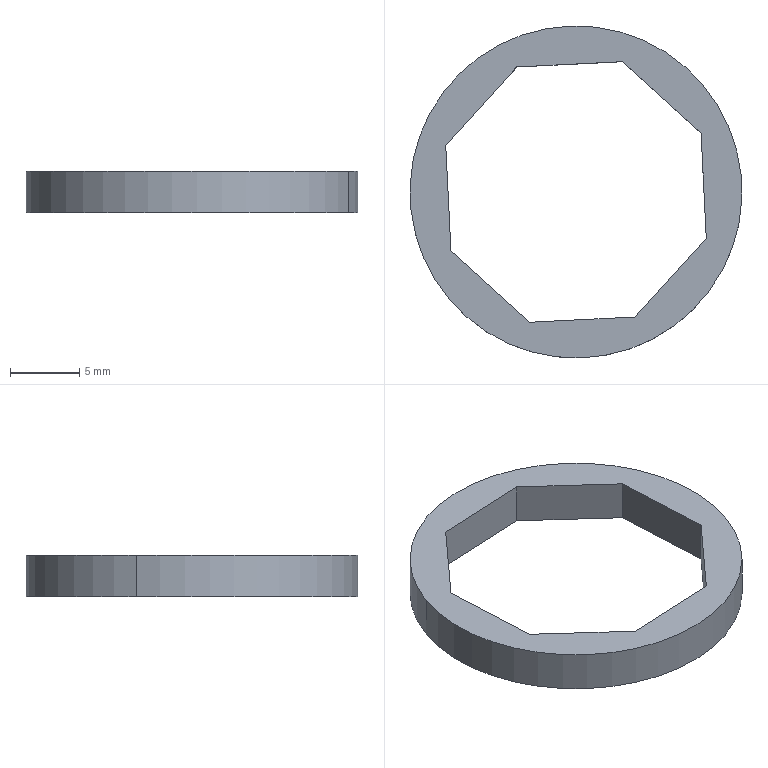Part | SolidWorks | features BaseBody 1 | 1 solid | 12 faces | box 24 x 24 x 3 mm | volume 508.64 mm3 | plane 10 | cylinder 2 | commonest cylinder face diameters 24 x2
STEP:
#1=CARTESIAN_POINT('',(-431.73,53.106,437.));
#2=VERTEX_POINT('',#1);
#3=CARTESIAN_POINT('',(-454.335,61.171,437.));
#4=VERTEX_POINT('',#3);
#5=CARTESIAN_POINT('',(-443.032,57.138,437.));
#6=DIRECTION('',(0.,0.,-1.));
#7=DIRECTION('',(0.9419,-0.336,0.));
#8=AXIS2_PLACEMENT_3D('',#5,#6,#7);
#9=CIRCLE('',#8,12.);
#10=EDGE_CURVE('',#2,#4,#9,.T.);
#11=ORIENTED_EDGE('',*,*,#10,.F.);
#12=CARTESIAN_POINT('',(-431.73,53.106,440.));
#13=VERTEX_POINT('',#12);
#14=CARTESIAN_POINT('',(-431.73,53.106,437.));
#15=DIRECTION('',(0.,0.,1.));
#16=VECTOR('',#15,1000.);
#17=LINE('',#14,#16);
#18=EDGE_CURVE('',#2,#13,#17,.T.);
#19=ORIENTED_EDGE('',*,*,#18,.T.);
#20=CARTESIAN_POINT('',(-454.335,61.171,440.));
#21=VERTEX_POINT('',#20);
#22=CARTESIAN_POINT('',(-443.032,57.138,440.));
#23=DIRECTION('',(0.,0.,-1.));
#24=DIRECTION('',(0.9419,-0.336,0.));
#25=AXIS2_PLACEMENT_3D('',#22,#23,#24);
#26=CIRCLE('',#25,12.);
#27=EDGE_CURVE('',#13,#21,#26,.T.);
#28=ORIENTED_EDGE('',*,*,#27,.T.);
#29=CARTESIAN_POINT('',(-454.335,61.171,437.));
#30=DIRECTION('',(0.,0.,1.));
#31=VECTOR('',#30,1000.);
#32=LINE('',#29,#31);
#33=EDGE_CURVE('',#4,#21,#32,.T.);
#34=ORIENTED_EDGE('',*,*,#33,.F.);
#35=EDGE_LOOP('',(#11,#19,#28,#34));
#36=FACE_OUTER_BOUND('',#35,.T.);
#37=CARTESIAN_POINT('',(-443.032,57.138,437.));
#38=DIRECTION('',(0.,0.,1.));
#39=DIRECTION('',(-0.9419,0.336,0.));
#40=AXIS2_PLACEMENT_3D('',#37,#38,#39);
#41=CYLINDRICAL_SURFACE('',#40,12.);
#42=ADVANCED_FACE('',(#36),#41,.T.);
#43=CARTESIAN_POINT('',(-443.032,57.138,437.));
#44=DIRECTION('',(0.,0.,-1.));
#45=DIRECTION('',(0.9419,-0.336,0.));
#46=AXIS2_PLACEMENT_3D('',#43,#44,#45);
#47=CIRCLE('',#46,12.);
#48=EDGE_CURVE('',#4,#2,#47,.T.);
#49=ORIENTED_EDGE('',*,*,#48,.T.);
#50=ORIENTED_EDGE('',*,*,#10,.T.);
#51=EDGE_LOOP('',(#49,#50));
#52=FACE_OUTER_BOUND('',#51,.T.);
#53=CARTESIAN_POINT('',(-433.614,53.778,437.));
#54=VERTEX_POINT('',#53);
#55=CARTESIAN_POINT('',(-438.748,48.102,437.));
#56=VERTEX_POINT('',#55);
#57=CARTESIAN_POINT('',(-433.614,53.778,437.));
#58=DIRECTION('',(-0.6709,-0.7416,0.));
#59=VECTOR('',#58,1000.);
#60=LINE('',#57,#59);
#61=EDGE_CURVE('',#54,#56,#60,.T.);
#62=ORIENTED_EDGE('',*,*,#61,.F.);
#63=CARTESIAN_POINT('',(-433.996,61.422,437.));
#64=VERTEX_POINT('',#63);
#65=CARTESIAN_POINT('',(-433.614,53.778,437.));
#66=DIRECTION('',(0.04998,-0.9987,0.));
#67=VECTOR('',#66,1000.);
#68=LINE('',#65,#67);
#69=EDGE_CURVE('',#64,#54,#68,.T.);
#70=ORIENTED_EDGE('',*,*,#69,.F.);
#71=CARTESIAN_POINT('',(-439.672,66.557,437.));
#72=VERTEX_POINT('',#71);
#73=CARTESIAN_POINT('',(-433.996,61.422,437.));
#74=DIRECTION('',(0.7416,-0.6709,0.));
#75=VECTOR('',#74,1000.);
#76=LINE('',#73,#75);
#77=EDGE_CURVE('',#72,#64,#76,.T.);
#78=ORIENTED_EDGE('',*,*,#77,.F.);
#79=CARTESIAN_POINT('',(-447.316,66.174,437.));
#80=VERTEX_POINT('',#79);
#81=CARTESIAN_POINT('',(-447.316,66.174,437.));
#82=DIRECTION('',(0.9987,0.04998,0.));
#83=VECTOR('',#82,1000.);
#84=LINE('',#81,#83);
#85=EDGE_CURVE('',#80,#72,#84,.T.);
#86=ORIENTED_EDGE('',*,*,#85,.F.);
#87=CARTESIAN_POINT('',(-452.451,60.499,437.));
#88=VERTEX_POINT('',#87);
#89=CARTESIAN_POINT('',(-452.451,60.499,437.));
#90=DIRECTION('',(0.6709,0.7416,0.));
#91=VECTOR('',#90,1000.);
#92=LINE('',#89,#91);
#93=EDGE_CURVE('',#88,#80,#92,.T.);
#94=ORIENTED_EDGE('',*,*,#93,.F.);
#95=CARTESIAN_POINT('',(-452.068,52.855,437.));
#96=VERTEX_POINT('',#95);
#97=CARTESIAN_POINT('',(-452.451,60.499,437.));
#98=DIRECTION('',(-0.04998,0.9987,0.));
#99=VECTOR('',#98,1000.);
#100=LINE('',#97,#99);
#101=EDGE_CURVE('',#96,#88,#100,.T.);
#102=ORIENTED_EDGE('',*,*,#101,.F.);
#103=CARTESIAN_POINT('',(-446.393,47.72,437.));
#104=VERTEX_POINT('',#103);
#105=CARTESIAN_POINT('',(-452.068,52.855,437.));
#106=DIRECTION('',(-0.7416,0.6709,0.));
#107=VECTOR('',#106,1000.);
#108=LINE('',#105,#107);
#109=EDGE_CURVE('',#104,#96,#108,.T.);
#110=ORIENTED_EDGE('',*,*,#109,.F.);
#111=CARTESIAN_POINT('',(-438.748,48.102,437.));
#112=DIRECTION('',(-0.9987,-0.04998,0.));
#113=VECTOR('',#112,1000.);
#114=LINE('',#111,#113);
#115=EDGE_CURVE('',#56,#104,#114,.T.);
#116=ORIENTED_EDGE('',*,*,#115,.F.);
#117=EDGE_LOOP('',(#62,#70,#78,#86,#94,#102,#110,#116));
#118=FACE_BOUND('',#117,.T.);
#119=CARTESIAN_POINT('',(-443.032,57.138,437.));
#120=DIRECTION('',(0.,0.,-1.));
#121=DIRECTION('',(0.9419,-0.336,0.));
#122=AXIS2_PLACEMENT_3D('',#119,#120,#121);
#123=PLANE('',#122);
#124=ADVANCED_FACE('',(#52,#118),#123,.T.);
#125=CARTESIAN_POINT('',(-443.032,57.138,440.));
#126=DIRECTION('',(0.,0.,-1.));
#127=DIRECTION('',(0.9419,-0.336,0.));
#128=AXIS2_PLACEMENT_3D('',#125,#126,#127);
#129=CIRCLE('',#128,12.);
#130=EDGE_CURVE('',#21,#13,#129,.T.);
#131=ORIENTED_EDGE('',*,*,#130,.F.);
#132=ORIENTED_EDGE('',*,*,#27,.F.);
#133=EDGE_LOOP('',(#131,#132));
#134=FACE_OUTER_BOUND('',#133,.T.);
#135=CARTESIAN_POINT('',(-433.996,61.422,440.));
#136=VERTEX_POINT('',#135);
#137=CARTESIAN_POINT('',(-433.614,53.778,440.));
#138=VERTEX_POINT('',#137);
#139=CARTESIAN_POINT('',(-433.614,53.778,440.));
#140=DIRECTION('',(0.04998,-0.9987,0.));
#141=VECTOR('',#140,1000.);
#142=LINE('',#139,#141);
#143=EDGE_CURVE('',#136,#138,#142,.T.);
#144=ORIENTED_EDGE('',*,*,#143,.T.);
#145=CARTESIAN_POINT('',(-438.748,48.102,440.));
#146=VERTEX_POINT('',#145);
#147=CARTESIAN_POINT('',(-433.614,53.778,440.));
#148=DIRECTION('',(-0.6709,-0.7416,0.));
#149=VECTOR('',#148,1000.);
#150=LINE('',#147,#149);
#151=EDGE_CURVE('',#138,#146,#150,.T.);
#152=ORIENTED_EDGE('',*,*,#151,.T.);
#153=CARTESIAN_POINT('',(-446.393,47.72,440.));
#154=VERTEX_POINT('',#153);
#155=CARTESIAN_POINT('',(-438.748,48.102,440.));
#156=DIRECTION('',(-0.9987,-0.04998,0.));
#157=VECTOR('',#156,1000.);
#158=LINE('',#155,#157);
#159=EDGE_CURVE('',#146,#154,#158,.T.);
#160=ORIENTED_EDGE('',*,*,#159,.T.);
#161=CARTESIAN_POINT('',(-452.068,52.855,440.));
#162=VERTEX_POINT('',#161);
#163=CARTESIAN_POINT('',(-452.068,52.855,440.));
#164=DIRECTION('',(-0.7416,0.6709,0.));
#165=VECTOR('',#164,1000.);
#166=LINE('',#163,#165);
#167=EDGE_CURVE('',#154,#162,#166,.T.);
#168=ORIENTED_EDGE('',*,*,#167,.T.);
#169=CARTESIAN_POINT('',(-452.451,60.499,440.));
#170=VERTEX_POINT('',#169);
#171=CARTESIAN_POINT('',(-452.451,60.499,440.));
#172=DIRECTION('',(-0.04998,0.9987,0.));
#173=VECTOR('',#172,1000.);
#174=LINE('',#171,#173);
#175=EDGE_CURVE('',#162,#170,#174,.T.);
#176=ORIENTED_EDGE('',*,*,#175,.T.);
#177=CARTESIAN_POINT('',(-447.316,66.174,440.));
#178=VERTEX_POINT('',#177);
#179=CARTESIAN_POINT('',(-452.451,60.499,440.));
#180=DIRECTION('',(0.6709,0.7416,0.));
#181=VECTOR('',#180,1000.);
#182=LINE('',#179,#181);
#183=EDGE_CURVE('',#170,#178,#182,.T.);
#184=ORIENTED_EDGE('',*,*,#183,.T.);
#185=CARTESIAN_POINT('',(-439.672,66.557,440.));
#186=VERTEX_POINT('',#185);
#187=CARTESIAN_POINT('',(-447.316,66.174,440.));
#188=DIRECTION('',(0.9987,0.04998,0.));
#189=VECTOR('',#188,1000.);
#190=LINE('',#187,#189);
#191=EDGE_CURVE('',#178,#186,#190,.T.);
#192=ORIENTED_EDGE('',*,*,#191,.T.);
#193=CARTESIAN_POINT('',(-433.996,61.422,440.));
#194=DIRECTION('',(0.7416,-0.6709,0.));
#195=VECTOR('',#194,1000.);
#196=LINE('',#193,#195);
#197=EDGE_CURVE('',#186,#136,#196,.T.);
#198=ORIENTED_EDGE('',*,*,#197,.T.);
#199=EDGE_LOOP('',(#144,#152,#160,#168,#176,#184,#192,#198));
#200=FACE_BOUND('',#199,.T.);
#201=CARTESIAN_POINT('',(-443.032,57.138,440.));
#202=DIRECTION('',(0.,0.,-1.));
#203=DIRECTION('',(0.9419,-0.336,0.));
#204=AXIS2_PLACEMENT_3D('',#201,#202,#203);
#205=PLANE('',#204);
#206=ADVANCED_FACE('',(#134,#200),#205,.F.);
#207=ORIENTED_EDGE('',*,*,#18,.F.);
#208=ORIENTED_EDGE('',*,*,#48,.F.);
#209=ORIENTED_EDGE('',*,*,#33,.T.);
#210=ORIENTED_EDGE('',*,*,#130,.T.);
#211=EDGE_LOOP('',(#207,#208,#209,#210));
#212=FACE_OUTER_BOUND('',#211,.T.);
#213=CARTESIAN_POINT('',(-443.032,57.138,437.));
#214=DIRECTION('',(0.,0.,1.));
#215=DIRECTION('',(-0.9419,0.336,0.));
#216=AXIS2_PLACEMENT_3D('',#213,#214,#215);
#217=CYLINDRICAL_SURFACE('',#216,12.);
#218=ADVANCED_FACE('',(#212),#217,.T.);
#219=ORIENTED_EDGE('',*,*,#143,.F.);
#220=CARTESIAN_POINT('',(-433.996,61.422,437.));
#221=DIRECTION('',(0.,0.,1.));
#222=VECTOR('',#221,1000.);
#223=LINE('',#220,#222);
#224=EDGE_CURVE('',#64,#136,#223,.T.);
#225=ORIENTED_EDGE('',*,*,#224,.F.);
#226=ORIENTED_EDGE('',*,*,#69,.T.);
#227=CARTESIAN_POINT('',(-433.614,53.778,437.));
#228=DIRECTION('',(0.,0.,1.));
#229=VECTOR('',#228,1000.);
#230=LINE('',#227,#229);
#231=EDGE_CURVE('',#54,#138,#230,.T.);
#232=ORIENTED_EDGE('',*,*,#231,.T.);
#233=EDGE_LOOP('',(#219,#225,#226,#232));
#234=FACE_OUTER_BOUND('',#233,.T.);
#235=CARTESIAN_POINT('',(-433.614,53.778,437.));
#236=DIRECTION('',(-0.9987,-0.04998,0.));
#237=DIRECTION('',(-0.04998,0.9987,0.));
#238=AXIS2_PLACEMENT_3D('',#235,#236,#237);
#239=PLANE('',#238);
#240=ADVANCED_FACE('',(#234),#239,.T.);
#241=ORIENTED_EDGE('',*,*,#151,.F.);
#242=ORIENTED_EDGE('',*,*,#231,.F.);
#243=ORIENTED_EDGE('',*,*,#61,.T.);
#244=CARTESIAN_POINT('',(-438.748,48.102,437.));
#245=DIRECTION('',(0.,0.,1.));
#246=VECTOR('',#245,1000.);
#247=LINE('',#244,#246);
#248=EDGE_CURVE('',#56,#146,#247,.T.);
#249=ORIENTED_EDGE('',*,*,#248,.T.);
#250=EDGE_LOOP('',(#241,#242,#243,#249));
#251=FACE_OUTER_BOUND('',#250,.T.);
#252=CARTESIAN_POINT('',(-433.614,53.778,437.));
#253=DIRECTION('',(-0.7416,0.6709,0.));
#254=DIRECTION('',(0.6709,0.7416,0.));
#255=AXIS2_PLACEMENT_3D('',#252,#253,#254);
#256=PLANE('',#255);
#257=ADVANCED_FACE('',(#251),#256,.T.);
#258=ORIENTED_EDGE('',*,*,#159,.F.);
#259=ORIENTED_EDGE('',*,*,#248,.F.);
#260=ORIENTED_EDGE('',*,*,#115,.T.);
#261=CARTESIAN_POINT('',(-446.393,47.72,437.));
#262=DIRECTION('',(0.,0.,1.));
#263=VECTOR('',#262,1000.);
#264=LINE('',#261,#263);
#265=EDGE_CURVE('',#104,#154,#264,.T.);
#266=ORIENTED_EDGE('',*,*,#265,.T.);
#267=EDGE_LOOP('',(#258,#259,#260,#266));
#268=FACE_OUTER_BOUND('',#267,.T.);
#269=CARTESIAN_POINT('',(-438.748,48.102,437.));
#270=DIRECTION('',(-0.04998,0.9987,0.));
#271=DIRECTION('',(0.9987,0.04998,0.));
#272=AXIS2_PLACEMENT_3D('',#269,#270,#271);
#273=PLANE('',#272);
#274=ADVANCED_FACE('',(#268),#273,.T.);
#275=ORIENTED_EDGE('',*,*,#167,.F.);
#276=ORIENTED_EDGE('',*,*,#265,.F.);
#277=ORIENTED_EDGE('',*,*,#109,.T.);
#278=CARTESIAN_POINT('',(-452.068,52.855,437.));
#279=DIRECTION('',(0.,0.,1.));
#280=VECTOR('',#279,1000.);
#281=LINE('',#278,#280);
#282=EDGE_CURVE('',#96,#162,#281,.T.);
#283=ORIENTED_EDGE('',*,*,#282,.T.);
#284=EDGE_LOOP('',(#275,#276,#277,#283));
#285=FACE_OUTER_BOUND('',#284,.T.);
#286=CARTESIAN_POINT('',(-452.068,52.855,437.));
#287=DIRECTION('',(0.6709,0.7416,0.));
#288=DIRECTION('',(0.7416,-0.6709,0.));
#289=AXIS2_PLACEMENT_3D('',#286,#287,#288);
#290=PLANE('',#289);
#291=ADVANCED_FACE('',(#285),#290,.T.);
#292=ORIENTED_EDGE('',*,*,#175,.F.);
#293=ORIENTED_EDGE('',*,*,#282,.F.);
#294=ORIENTED_EDGE('',*,*,#101,.T.);
#295=CARTESIAN_POINT('',(-452.451,60.499,437.));
#296=DIRECTION('',(0.,0.,1.));
#297=VECTOR('',#296,1000.);
#298=LINE('',#295,#297);
#299=EDGE_CURVE('',#88,#170,#298,.T.);
#300=ORIENTED_EDGE('',*,*,#299,.T.);
#301=EDGE_LOOP('',(#292,#293,#294,#300));
#302=FACE_OUTER_BOUND('',#301,.T.);
#303=CARTESIAN_POINT('',(-452.451,60.499,437.));
#304=DIRECTION('',(0.9987,0.04998,0.));
#305=DIRECTION('',(0.04998,-0.9987,0.));
#306=AXIS2_PLACEMENT_3D('',#303,#304,#305);
#307=PLANE('',#306);
#308=ADVANCED_FACE('',(#302),#307,.T.);
#309=ORIENTED_EDGE('',*,*,#183,.F.);
#310=ORIENTED_EDGE('',*,*,#299,.F.);
#311=ORIENTED_EDGE('',*,*,#93,.T.);
#312=CARTESIAN_POINT('',(-447.316,66.174,437.));
#313=DIRECTION('',(0.,0.,1.));
#314=VECTOR('',#313,1000.);
#315=LINE('',#312,#314);
#316=EDGE_CURVE('',#80,#178,#315,.T.);
#317=ORIENTED_EDGE('',*,*,#316,.T.);
#318=EDGE_LOOP('',(#309,#310,#311,#317));
#319=FACE_OUTER_BOUND('',#318,.T.);
#320=CARTESIAN_POINT('',(-452.451,60.499,437.));
#321=DIRECTION('',(0.7416,-0.6709,0.));
#322=DIRECTION('',(-0.6709,-0.7416,0.));
#323=AXIS2_PLACEMENT_3D('',#320,#321,#322);
#324=PLANE('',#323);
#325=ADVANCED_FACE('',(#319),#324,.T.);
#326=ORIENTED_EDGE('',*,*,#191,.F.);
#327=ORIENTED_EDGE('',*,*,#316,.F.);
#328=ORIENTED_EDGE('',*,*,#85,.T.);
#329=CARTESIAN_POINT('',(-439.672,66.557,437.));
#330=DIRECTION('',(0.,0.,1.));
#331=VECTOR('',#330,1000.);
#332=LINE('',#329,#331);
#333=EDGE_CURVE('',#72,#186,#332,.T.);
#334=ORIENTED_EDGE('',*,*,#333,.T.);
#335=EDGE_LOOP('',(#326,#327,#328,#334));
#336=FACE_OUTER_BOUND('',#335,.T.);
#337=CARTESIAN_POINT('',(-447.316,66.174,437.));
#338=DIRECTION('',(0.04998,-0.9987,0.));
#339=DIRECTION('',(-0.9987,-0.04998,0.));
#340=AXIS2_PLACEMENT_3D('',#337,#338,#339);
#341=PLANE('',#340);
#342=ADVANCED_FACE('',(#336),#341,.T.);
#343=ORIENTED_EDGE('',*,*,#197,.F.);
#344=ORIENTED_EDGE('',*,*,#333,.F.);
#345=ORIENTED_EDGE('',*,*,#77,.T.);
#346=ORIENTED_EDGE('',*,*,#224,.T.);
#347=EDGE_LOOP('',(#343,#344,#345,#346));
#348=FACE_OUTER_BOUND('',#347,.T.);
#349=CARTESIAN_POINT('',(-433.996,61.422,437.));
#350=DIRECTION('',(-0.6709,-0.7416,0.));
#351=DIRECTION('',(-0.7416,0.6709,0.));
#352=AXIS2_PLACEMENT_3D('',#349,#350,#351);
#353=PLANE('',#352);
#354=ADVANCED_FACE('',(#348),#353,.T.);
#355=CLOSED_SHELL('',(#42,#124,#206,#218,#240,#257,#274,#291,#308,#325,#342,#354));
#356=MANIFOLD_SOLID_BREP('',#355);
#357=CARTESIAN_POINT('',(0.,0.,0.));
#358=DIRECTION('',(0.,0.,1.));
#359=DIRECTION('',(1.,0.,0.));
#360=AXIS2_PLACEMENT_3D('',#357,#358,#359);
#361=(LENGTH_UNIT()NAMED_UNIT(*)SI_UNIT(.MILLI.,.METRE.));
#362=UNCERTAINTY_MEASURE_WITH_UNIT(LENGTH_MEASURE(0.00001),#361,'','');
#363=(NAMED_UNIT(*)PLANE_ANGLE_UNIT()SI_UNIT($,.RADIAN.));
#364=(NAMED_UNIT(*)SI_UNIT($,.STERADIAN.)SOLID_ANGLE_UNIT());
#365=(GEOMETRIC_REPRESENTATION_CONTEXT(3)GLOBAL_UNCERTAINTY_ASSIGNED_CONTEXT((#362))GLOBAL_UNIT_ASSIGNED_CONTEXT((#361,#363,#364))REPRESENTATION_CONTEXT('',''));
#366=ADVANCED_BREP_SHAPE_REPRESENTATION('',(#356,#360),#365);